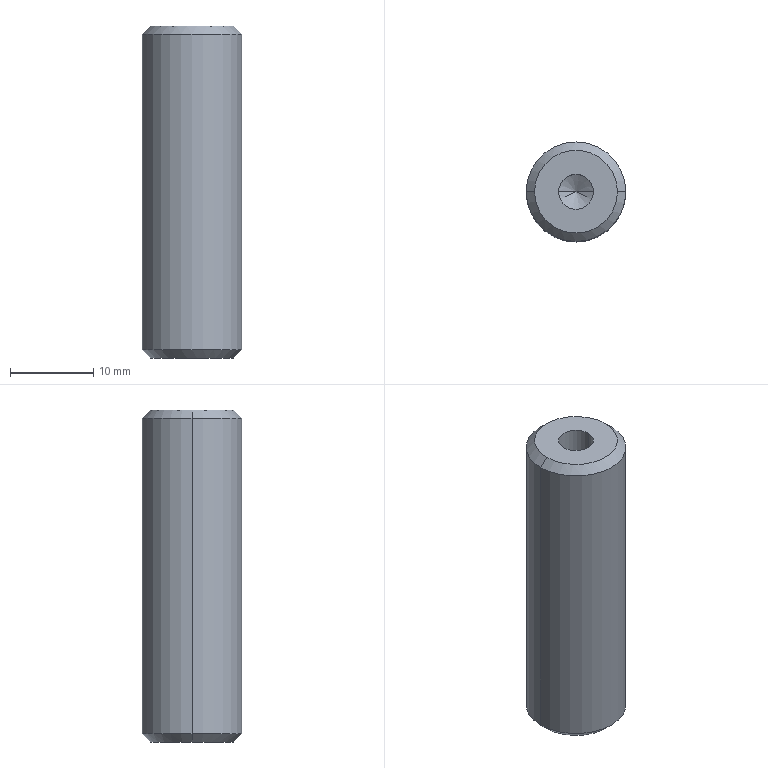Part | STEP file | PSFGT12-40-M5 | 1 solid | 12 faces | box 12 x 12 x 40 mm | volume 4311 mm3 | cone 6 | cylinder 4 | plane 2 | commonest cylinder face diameters 4.2 x2 12 x2
STEP:
#1=CARTESIAN_POINT('',(0.,0.,0.));
#2=DIRECTION('',(0.,0.,1.));
#3=DIRECTION('',(1.,0.,0.));
#4=AXIS2_PLACEMENT_3D('',#1,#2,#3);
#5=CARTESIAN_POINT('',(2.1,0.,27.6));
#6=VERTEX_POINT('',#5);
#7=CARTESIAN_POINT('',(2.1,0.,40.));
#8=VERTEX_POINT('',#7);
#9=CARTESIAN_POINT('',(2.1,0.,40.));
#10=DIRECTION('',(0.,0.,1.));
#11=VECTOR('',#10,1.);
#12=LINE('',#9,#11);
#13=CARTESIAN_POINT('',(0.,0.,40.));
#14=DIRECTION('',(0.,0.,1.));
#15=DIRECTION('',(1.,0.,0.));
#16=AXIS2_PLACEMENT_3D('',#13,#14,#15);
#17=CYLINDRICAL_SURFACE('',#16,2.1);
#18=CARTESIAN_POINT('',(6.283,0.));
#19=DIRECTION('',(0.,1.));
#20=VECTOR('',#19,1.);
#21=LINE('',#18,#20);
#22=(GEOMETRIC_REPRESENTATION_CONTEXT(2)PARAMETRIC_REPRESENTATION_CONTEXT()REPRESENTATION_CONTEXT('',''));
#23=DEFINITIONAL_REPRESENTATION('',(#21),#22);
#24=PCURVE('',#17,#23);
#25=CARTESIAN_POINT('',(0.,0.,40.));
#26=DIRECTION('',(0.,0.,1.));
#27=DIRECTION('',(1.,0.,0.));
#28=AXIS2_PLACEMENT_3D('',#25,#26,#27);
#29=CYLINDRICAL_SURFACE('',#28,2.1);
#30=CARTESIAN_POINT('',(0.,0.));
#31=DIRECTION('',(0.,1.));
#32=VECTOR('',#31,1.);
#33=LINE('',#30,#32);
#34=(GEOMETRIC_REPRESENTATION_CONTEXT(2)PARAMETRIC_REPRESENTATION_CONTEXT()REPRESENTATION_CONTEXT('',''));
#35=DEFINITIONAL_REPRESENTATION('',(#33),#34);
#36=PCURVE('',#29,#35);
#37=SURFACE_CURVE('',#12,(#24,#36),.PCURVE_S1.);
#38=EDGE_CURVE('',#6,#8,#37,.T.);
#39=ORIENTED_EDGE('',*,*,#38,.T.);
#40=CARTESIAN_POINT('',(-2.1,0.,40.));
#41=VERTEX_POINT('',#40);
#42=CARTESIAN_POINT('',(0.,0.,40.));
#43=DIRECTION('',(0.,0.,1.));
#44=DIRECTION('',(1.,0.,0.));
#45=AXIS2_PLACEMENT_3D('',#42,#43,#44);
#46=CIRCLE('',#45,2.1);
#47=CARTESIAN_POINT('',(0.,0.));
#48=DIRECTION('',(1.,0.));
#49=VECTOR('',#48,1.);
#50=LINE('',#47,#49);
#51=(GEOMETRIC_REPRESENTATION_CONTEXT(2)PARAMETRIC_REPRESENTATION_CONTEXT()REPRESENTATION_CONTEXT('',''));
#52=DEFINITIONAL_REPRESENTATION('',(#50),#51);
#53=PCURVE('',#17,#52);
#54=CARTESIAN_POINT('',(0.,0.,40.));
#55=DIRECTION('',(0.,0.,1.));
#56=DIRECTION('',(1.,0.,0.));
#57=AXIS2_PLACEMENT_3D('',#54,#55,#56);
#58=PLANE('',#57);
#59=CARTESIAN_POINT('',(0.,0.));
#60=DIRECTION('',(1.,0.));
#61=AXIS2_PLACEMENT_2D('',#59,#60);
#62=CIRCLE('',#61,2.1);
#63=(GEOMETRIC_REPRESENTATION_CONTEXT(2)PARAMETRIC_REPRESENTATION_CONTEXT()REPRESENTATION_CONTEXT('',''));
#64=DEFINITIONAL_REPRESENTATION('',(#62),#63);
#65=PCURVE('',#58,#64);
#66=SURFACE_CURVE('',#46,(#53,#65),.PCURVE_S1.);
#67=EDGE_CURVE('',#41,#8,#66,.T.);
#68=ORIENTED_EDGE('',*,*,#67,.F.);
#69=CARTESIAN_POINT('',(-2.1,0.,27.6));
#70=VERTEX_POINT('',#69);
#71=CARTESIAN_POINT('',(-2.1,0.,40.));
#72=DIRECTION('',(0.,0.,1.));
#73=VECTOR('',#72,1.);
#74=LINE('',#71,#73);
#75=CARTESIAN_POINT('',(3.142,0.));
#76=DIRECTION('',(0.,1.));
#77=VECTOR('',#76,1.);
#78=LINE('',#75,#77);
#79=(GEOMETRIC_REPRESENTATION_CONTEXT(2)PARAMETRIC_REPRESENTATION_CONTEXT()REPRESENTATION_CONTEXT('',''));
#80=DEFINITIONAL_REPRESENTATION('',(#78),#79);
#81=PCURVE('',#17,#80);
#82=CARTESIAN_POINT('',(3.142,0.));
#83=DIRECTION('',(0.,1.));
#84=VECTOR('',#83,1.);
#85=LINE('',#82,#84);
#86=(GEOMETRIC_REPRESENTATION_CONTEXT(2)PARAMETRIC_REPRESENTATION_CONTEXT()REPRESENTATION_CONTEXT('',''));
#87=DEFINITIONAL_REPRESENTATION('',(#85),#86);
#88=PCURVE('',#29,#87);
#89=SURFACE_CURVE('',#74,(#81,#88),.PCURVE_S1.);
#90=EDGE_CURVE('',#70,#41,#89,.T.);
#91=ORIENTED_EDGE('',*,*,#90,.F.);
#92=CARTESIAN_POINT('',(0.,0.,27.6));
#93=DIRECTION('',(0.,0.,1.));
#94=DIRECTION('',(1.,0.,0.));
#95=AXIS2_PLACEMENT_3D('',#92,#93,#94);
#96=CIRCLE('',#95,2.1);
#97=CARTESIAN_POINT('',(0.,-12.4));
#98=DIRECTION('',(1.,0.));
#99=VECTOR('',#98,1.);
#100=LINE('',#97,#99);
#101=(GEOMETRIC_REPRESENTATION_CONTEXT(2)PARAMETRIC_REPRESENTATION_CONTEXT()REPRESENTATION_CONTEXT('',''));
#102=DEFINITIONAL_REPRESENTATION('',(#100),#101);
#103=PCURVE('',#17,#102);
#104=CARTESIAN_POINT('',(0.,0.,27.6));
#105=DIRECTION('',(0.,0.,1.));
#106=DIRECTION('',(1.,0.,0.));
#107=AXIS2_PLACEMENT_3D('',#104,#105,#106);
#108=CONICAL_SURFACE('',#107,2.1,1.03);
#109=CARTESIAN_POINT('',(0.,0.));
#110=DIRECTION('',(1.,0.));
#111=VECTOR('',#110,1.);
#112=LINE('',#109,#111);
#113=(GEOMETRIC_REPRESENTATION_CONTEXT(2)PARAMETRIC_REPRESENTATION_CONTEXT()REPRESENTATION_CONTEXT('',''));
#114=DEFINITIONAL_REPRESENTATION('',(#112),#113);
#115=PCURVE('',#108,#114);
#116=SURFACE_CURVE('',#96,(#103,#115),.PCURVE_S1.);
#117=EDGE_CURVE('',#70,#6,#116,.T.);
#118=ORIENTED_EDGE('',*,*,#117,.T.);
#119=EDGE_LOOP('',(#39,#68,#91,#118));
#120=FACE_BOUND('',#119,.F.);
#121=ADVANCED_FACE('',(#120),#17,.F.);
#122=ORIENTED_EDGE('',*,*,#117,.F.);
#123=CARTESIAN_POINT('',(0.,0.,26.338));
#124=VERTEX_POINT('',#123);
#125=CARTESIAN_POINT('',(-2.1,0.,27.6));
#126=DIRECTION('',(-0.8572,0.,0.515));
#127=VECTOR('',#126,1.);
#128=LINE('',#125,#127);
#129=CARTESIAN_POINT('',(3.142,0.));
#130=DIRECTION('',(0.,1.));
#131=VECTOR('',#130,1.);
#132=LINE('',#129,#131);
#133=(GEOMETRIC_REPRESENTATION_CONTEXT(2)PARAMETRIC_REPRESENTATION_CONTEXT()REPRESENTATION_CONTEXT('',''));
#134=DEFINITIONAL_REPRESENTATION('',(#132),#133);
#135=PCURVE('',#108,#134);
#136=CARTESIAN_POINT('',(0.,0.,27.6));
#137=DIRECTION('',(0.,0.,1.));
#138=DIRECTION('',(1.,0.,0.));
#139=AXIS2_PLACEMENT_3D('',#136,#137,#138);
#140=CONICAL_SURFACE('',#139,2.1,1.03);
#141=CARTESIAN_POINT('',(3.142,0.));
#142=DIRECTION('',(0.,1.));
#143=VECTOR('',#142,1.);
#144=LINE('',#141,#143);
#145=(GEOMETRIC_REPRESENTATION_CONTEXT(2)PARAMETRIC_REPRESENTATION_CONTEXT()REPRESENTATION_CONTEXT('',''));
#146=DEFINITIONAL_REPRESENTATION('',(#144),#145);
#147=PCURVE('',#140,#146);
#148=SURFACE_CURVE('',#128,(#135,#147),.PCURVE_S1.);
#149=EDGE_CURVE('',#124,#70,#148,.T.);
#150=ORIENTED_EDGE('',*,*,#149,.F.);
#151=CARTESIAN_POINT('',(2.1,0.,27.6));
#152=DIRECTION('',(0.8572,0.,0.515));
#153=VECTOR('',#152,1.);
#154=LINE('',#151,#153);
#155=CARTESIAN_POINT('',(6.283,-1.262));
#156=CARTESIAN_POINT('',(6.283,-1.243));
#157=CARTESIAN_POINT('',(6.283,-1.204));
#158=CARTESIAN_POINT('',(6.283,-1.147));
#159=CARTESIAN_POINT('',(6.283,-1.09));
#160=CARTESIAN_POINT('',(6.283,-1.032));
#161=CARTESIAN_POINT('',(6.283,-0.975));
#162=CARTESIAN_POINT('',(6.283,-0.9177));
#163=CARTESIAN_POINT('',(6.283,-0.8603));
#164=CARTESIAN_POINT('',(6.283,-0.803));
#165=CARTESIAN_POINT('',(6.283,-0.7456));
#166=CARTESIAN_POINT('',(6.283,-0.6883));
#167=CARTESIAN_POINT('',(6.283,-0.6309));
#168=CARTESIAN_POINT('',(6.283,-0.5735));
#169=CARTESIAN_POINT('',(6.283,-0.5162));
#170=CARTESIAN_POINT('',(6.283,-0.4588));
#171=CARTESIAN_POINT('',(6.283,-0.4015));
#172=CARTESIAN_POINT('',(6.283,-0.3441));
#173=CARTESIAN_POINT('',(6.283,-0.2868));
#174=CARTESIAN_POINT('',(6.283,-0.2294));
#175=CARTESIAN_POINT('',(6.283,-0.1721));
#176=CARTESIAN_POINT('',(6.283,-0.1147));
#177=CARTESIAN_POINT('',(6.283,-0.05735));
#178=CARTESIAN_POINT('',(6.283,-0.01912));
#179=CARTESIAN_POINT('',(6.283,0.));
#180=B_SPLINE_CURVE_WITH_KNOTS('',3,(#155,#156,#157,#158,#159,#160,#161,#162,#163,#164,#165,#166,#167,#168,#169,#170,#171,#172,#173,#174,#175,#176,#177,#178,#179),.UNSPECIFIED.,.F.,.F.,(4,1,1,1,1,1,1,1,1,1,1,1,1,1,1,1,1,1,1,1,1,1,4),(-2.45,-2.339,-2.227,-2.116,-2.004,-1.893,-1.782,-1.67,-1.559,-1.448,-1.336,-1.225,-1.114,-1.002,-0.8909,-0.7795,-0.6682,-0.5568,-0.4454,-0.3341,-0.2227,-0.1114,0.),.UNSPECIFIED.);
#181=(GEOMETRIC_REPRESENTATION_CONTEXT(2)PARAMETRIC_REPRESENTATION_CONTEXT()REPRESENTATION_CONTEXT('',''));
#182=DEFINITIONAL_REPRESENTATION('',(#180),#181);
#183=PCURVE('',#108,#182);
#184=CARTESIAN_POINT('',(0.,-1.262));
#185=CARTESIAN_POINT('',(0.,-1.243));
#186=CARTESIAN_POINT('',(0.,-1.204));
#187=CARTESIAN_POINT('',(0.,-1.147));
#188=CARTESIAN_POINT('',(0.,-1.09));
#189=CARTESIAN_POINT('',(0.,-1.032));
#190=CARTESIAN_POINT('',(0.,-0.975));
#191=CARTESIAN_POINT('',(0.,-0.9177));
#192=CARTESIAN_POINT('',(0.,-0.8603));
#193=CARTESIAN_POINT('',(0.,-0.803));
#194=CARTESIAN_POINT('',(0.,-0.7456));
#195=CARTESIAN_POINT('',(0.,-0.6883));
#196=CARTESIAN_POINT('',(0.,-0.6309));
#197=CARTESIAN_POINT('',(0.,-0.5735));
#198=CARTESIAN_POINT('',(0.,-0.5162));
#199=CARTESIAN_POINT('',(0.,-0.4588));
#200=CARTESIAN_POINT('',(0.,-0.4015));
#201=CARTESIAN_POINT('',(0.,-0.3441));
#202=CARTESIAN_POINT('',(0.,-0.2868));
#203=CARTESIAN_POINT('',(0.,-0.2294));
#204=CARTESIAN_POINT('',(0.,-0.1721));
#205=CARTESIAN_POINT('',(0.,-0.1147));
#206=CARTESIAN_POINT('',(0.,-0.05735));
#207=CARTESIAN_POINT('',(0.,-0.01912));
#208=CARTESIAN_POINT('',(0.,0.));
#209=B_SPLINE_CURVE_WITH_KNOTS('',3,(#184,#185,#186,#187,#188,#189,#190,#191,#192,#193,#194,#195,#196,#197,#198,#199,#200,#201,#202,#203,#204,#205,#206,#207,#208),.UNSPECIFIED.,.F.,.F.,(4,1,1,1,1,1,1,1,1,1,1,1,1,1,1,1,1,1,1,1,1,1,4),(-2.45,-2.339,-2.227,-2.116,-2.004,-1.893,-1.782,-1.67,-1.559,-1.448,-1.336,-1.225,-1.114,-1.002,-0.8909,-0.7795,-0.6682,-0.5568,-0.4454,-0.3341,-0.2227,-0.1114,0.),.UNSPECIFIED.);
#210=(GEOMETRIC_REPRESENTATION_CONTEXT(2)PARAMETRIC_REPRESENTATION_CONTEXT()REPRESENTATION_CONTEXT('',''));
#211=DEFINITIONAL_REPRESENTATION('',(#209),#210);
#212=PCURVE('',#140,#211);
#213=SURFACE_CURVE('',#154,(#183,#212),.PCURVE_S1.);
#214=EDGE_CURVE('',#124,#6,#213,.T.);
#215=ORIENTED_EDGE('',*,*,#214,.T.);
#216=EDGE_LOOP('',(#122,#150,#215));
#217=FACE_BOUND('',#216,.F.);
#218=ADVANCED_FACE('',(#217),#108,.F.);
#219=CARTESIAN_POINT('',(5.,0.,40.));
#220=VERTEX_POINT('',#219);
#221=CARTESIAN_POINT('',(-5.,0.,40.));
#222=VERTEX_POINT('',#221);
#223=CARTESIAN_POINT('',(0.,0.,40.));
#224=DIRECTION('',(0.,0.,1.));
#225=DIRECTION('',(1.,0.,0.));
#226=AXIS2_PLACEMENT_3D('',#223,#224,#225);
#227=CIRCLE('',#226,5.);
#228=CARTESIAN_POINT('',(0.,0.,40.));
#229=DIRECTION('',(0.,0.,-1.));
#230=DIRECTION('',(-1.,0.,0.));
#231=AXIS2_PLACEMENT_3D('',#228,#229,#230);
#232=CONICAL_SURFACE('',#231,5.,0.7854);
#233=CARTESIAN_POINT('',(3.142,0.));
#234=DIRECTION('',(-1.,0.));
#235=VECTOR('',#234,1.);
#236=LINE('',#233,#235);
#237=(GEOMETRIC_REPRESENTATION_CONTEXT(2)PARAMETRIC_REPRESENTATION_CONTEXT()REPRESENTATION_CONTEXT('',''));
#238=DEFINITIONAL_REPRESENTATION('',(#236),#237);
#239=PCURVE('',#232,#238);
#240=CARTESIAN_POINT('',(0.,0.));
#241=DIRECTION('',(1.,0.));
#242=AXIS2_PLACEMENT_2D('',#240,#241);
#243=CIRCLE('',#242,5.);
#244=(GEOMETRIC_REPRESENTATION_CONTEXT(2)PARAMETRIC_REPRESENTATION_CONTEXT()REPRESENTATION_CONTEXT('',''));
#245=DEFINITIONAL_REPRESENTATION('',(#243),#244);
#246=PCURVE('',#58,#245);
#247=SURFACE_CURVE('',#227,(#239,#246),.PCURVE_S1.);
#248=EDGE_CURVE('',#220,#222,#247,.T.);
#249=ORIENTED_EDGE('',*,*,#248,.F.);
#250=CARTESIAN_POINT('',(6.,0.,39.));
#251=VERTEX_POINT('',#250);
#252=CARTESIAN_POINT('',(5.,0.,40.));
#253=DIRECTION('',(0.7071,0.,-0.7071));
#254=VECTOR('',#253,1.);
#255=LINE('',#252,#254);
#256=CARTESIAN_POINT('',(3.142,0.));
#257=DIRECTION('',(0.,1.));
#258=VECTOR('',#257,1.);
#259=LINE('',#256,#258);
#260=(GEOMETRIC_REPRESENTATION_CONTEXT(2)PARAMETRIC_REPRESENTATION_CONTEXT()REPRESENTATION_CONTEXT('',''));
#261=DEFINITIONAL_REPRESENTATION('',(#259),#260);
#262=PCURVE('',#232,#261);
#263=CARTESIAN_POINT('',(0.,0.,40.));
#264=DIRECTION('',(0.,0.,-1.));
#265=DIRECTION('',(-1.,0.,0.));
#266=AXIS2_PLACEMENT_3D('',#263,#264,#265);
#267=CONICAL_SURFACE('',#266,5.,0.7854);
#268=CARTESIAN_POINT('',(3.142,0.));
#269=DIRECTION('',(0.,1.));
#270=VECTOR('',#269,1.);
#271=LINE('',#268,#270);
#272=(GEOMETRIC_REPRESENTATION_CONTEXT(2)PARAMETRIC_REPRESENTATION_CONTEXT()REPRESENTATION_CONTEXT('',''));
#273=DEFINITIONAL_REPRESENTATION('',(#271),#272);
#274=PCURVE('',#267,#273);
#275=SURFACE_CURVE('',#255,(#262,#274),.PCURVE_S1.);
#276=EDGE_CURVE('',#220,#251,#275,.T.);
#277=ORIENTED_EDGE('',*,*,#276,.T.);
#278=CARTESIAN_POINT('',(-6.,0.,39.));
#279=VERTEX_POINT('',#278);
#280=CARTESIAN_POINT('',(0.,0.,39.));
#281=DIRECTION('',(0.,0.,-1.));
#282=DIRECTION('',(1.,0.,0.));
#283=AXIS2_PLACEMENT_3D('',#280,#281,#282);
#284=CIRCLE('',#283,6.);
#285=CARTESIAN_POINT('',(-3.142,1.));
#286=DIRECTION('',(1.,0.));
#287=VECTOR('',#286,1.);
#288=LINE('',#285,#287);
#289=(GEOMETRIC_REPRESENTATION_CONTEXT(2)PARAMETRIC_REPRESENTATION_CONTEXT()REPRESENTATION_CONTEXT('',''));
#290=DEFINITIONAL_REPRESENTATION('',(#288),#289);
#291=PCURVE('',#232,#290);
#292=CARTESIAN_POINT('',(0.,0.,40.));
#293=DIRECTION('',(0.,0.,-1.));
#294=DIRECTION('',(-1.,0.,0.));
#295=AXIS2_PLACEMENT_3D('',#292,#293,#294);
#296=CYLINDRICAL_SURFACE('',#295,6.);
#297=CARTESIAN_POINT('',(-3.142,1.));
#298=DIRECTION('',(1.,0.));
#299=VECTOR('',#298,1.);
#300=LINE('',#297,#299);
#301=(GEOMETRIC_REPRESENTATION_CONTEXT(2)PARAMETRIC_REPRESENTATION_CONTEXT()REPRESENTATION_CONTEXT('',''));
#302=DEFINITIONAL_REPRESENTATION('',(#300),#301);
#303=PCURVE('',#296,#302);
#304=SURFACE_CURVE('',#284,(#291,#303),.PCURVE_S1.);
#305=EDGE_CURVE('',#279,#251,#304,.T.);
#306=ORIENTED_EDGE('',*,*,#305,.F.);
#307=CARTESIAN_POINT('',(-5.,0.,40.));
#308=DIRECTION('',(-0.7071,0.,-0.7071));
#309=VECTOR('',#308,1.);
#310=LINE('',#307,#309);
#311=CARTESIAN_POINT('',(0.,0.));
#312=DIRECTION('',(0.,1.));
#313=VECTOR('',#312,1.);
#314=LINE('',#311,#313);
#315=(GEOMETRIC_REPRESENTATION_CONTEXT(2)PARAMETRIC_REPRESENTATION_CONTEXT()REPRESENTATION_CONTEXT('',''));
#316=DEFINITIONAL_REPRESENTATION('',(#314),#315);
#317=PCURVE('',#232,#316);
#318=CARTESIAN_POINT('',(6.283,0.));
#319=DIRECTION('',(0.,1.));
#320=VECTOR('',#319,1.);
#321=LINE('',#318,#320);
#322=(GEOMETRIC_REPRESENTATION_CONTEXT(2)PARAMETRIC_REPRESENTATION_CONTEXT()REPRESENTATION_CONTEXT('',''));
#323=DEFINITIONAL_REPRESENTATION('',(#321),#322);
#324=PCURVE('',#267,#323);
#325=SURFACE_CURVE('',#310,(#317,#324),.PCURVE_S1.);
#326=EDGE_CURVE('',#222,#279,#325,.T.);
#327=ORIENTED_EDGE('',*,*,#326,.F.);
#328=EDGE_LOOP('',(#249,#277,#306,#327));
#329=FACE_BOUND('',#328,.T.);
#330=ADVANCED_FACE('',(#329),#232,.T.);
#331=CARTESIAN_POINT('',(-5.,0.,0.));
#332=VERTEX_POINT('',#331);
#333=CARTESIAN_POINT('',(5.,0.,0.));
#334=VERTEX_POINT('',#333);
#335=CARTESIAN_POINT('',(0.,0.,0.));
#336=DIRECTION('',(0.,0.,-1.));
#337=DIRECTION('',(1.,0.,0.));
#338=AXIS2_PLACEMENT_3D('',#335,#336,#337);
#339=CIRCLE('',#338,5.);
#340=CARTESIAN_POINT('',(0.,0.,1.));
#341=DIRECTION('',(0.,0.,1.));
#342=DIRECTION('',(1.,0.,0.));
#343=AXIS2_PLACEMENT_3D('',#340,#341,#342);
#344=CONICAL_SURFACE('',#343,6.,0.7854);
#345=CARTESIAN_POINT('',(6.283,-1.));
#346=DIRECTION('',(-1.,0.));
#347=VECTOR('',#346,1.);
#348=LINE('',#345,#347);
#349=(GEOMETRIC_REPRESENTATION_CONTEXT(2)PARAMETRIC_REPRESENTATION_CONTEXT()REPRESENTATION_CONTEXT('',''));
#350=DEFINITIONAL_REPRESENTATION('',(#348),#349);
#351=PCURVE('',#344,#350);
#352=CARTESIAN_POINT('',(0.,0.,0.));
#353=DIRECTION('',(0.,0.,1.));
#354=DIRECTION('',(1.,0.,0.));
#355=AXIS2_PLACEMENT_3D('',#352,#353,#354);
#356=PLANE('',#355);
#357=CARTESIAN_POINT('',(5.,0.));
#358=CARTESIAN_POINT('',(5.,-8.66));
#359=CARTESIAN_POINT('',(-2.5,-4.33));
#360=CARTESIAN_POINT('',(-10.,0.));
#361=CARTESIAN_POINT('',(-2.5,4.33));
#362=CARTESIAN_POINT('',(5.,8.66));
#363=CARTESIAN_POINT('',(5.,0.));
#364=(BOUNDED_CURVE()B_SPLINE_CURVE(2,(#357,#358,#359,#360,#361,#362,#363),.UNSPECIFIED.,.T.,.F.)B_SPLINE_CURVE_WITH_KNOTS((1,2,2,2,2,1),(-2.094,0.,2.094,4.189,6.283,8.378),.UNSPECIFIED.)CURVE()GEOMETRIC_REPRESENTATION_ITEM()RATIONAL_B_SPLINE_CURVE((1.,0.5,1.,0.5,1.,0.5,1.))REPRESENTATION_ITEM(''));
#365=(GEOMETRIC_REPRESENTATION_CONTEXT(2)PARAMETRIC_REPRESENTATION_CONTEXT()REPRESENTATION_CONTEXT('',''));
#366=DEFINITIONAL_REPRESENTATION('',(#364),#365);
#367=PCURVE('',#356,#366);
#368=SURFACE_CURVE('',#339,(#351,#367),.PCURVE_S1.);
#369=EDGE_CURVE('',#332,#334,#368,.T.);
#370=ORIENTED_EDGE('',*,*,#369,.F.);
#371=CARTESIAN_POINT('',(-6.,0.,1.));
#372=VERTEX_POINT('',#371);
#373=CARTESIAN_POINT('',(-6.,0.,1.));
#374=DIRECTION('',(-0.7071,0.,0.7071));
#375=VECTOR('',#374,1.);
#376=LINE('',#373,#375);
#377=CARTESIAN_POINT('',(3.142,0.));
#378=DIRECTION('',(0.,1.));
#379=VECTOR('',#378,1.);
#380=LINE('',#377,#379);
#381=(GEOMETRIC_REPRESENTATION_CONTEXT(2)PARAMETRIC_REPRESENTATION_CONTEXT()REPRESENTATION_CONTEXT('',''));
#382=DEFINITIONAL_REPRESENTATION('',(#380),#381);
#383=PCURVE('',#344,#382);
#384=CARTESIAN_POINT('',(0.,0.,1.));
#385=DIRECTION('',(0.,0.,1.));
#386=DIRECTION('',(1.,0.,0.));
#387=AXIS2_PLACEMENT_3D('',#384,#385,#386);
#388=CONICAL_SURFACE('',#387,6.,0.7854);
#389=CARTESIAN_POINT('',(3.142,0.));
#390=DIRECTION('',(0.,1.));
#391=VECTOR('',#390,1.);
#392=LINE('',#389,#391);
#393=(GEOMETRIC_REPRESENTATION_CONTEXT(2)PARAMETRIC_REPRESENTATION_CONTEXT()REPRESENTATION_CONTEXT('',''));
#394=DEFINITIONAL_REPRESENTATION('',(#392),#393);
#395=PCURVE('',#388,#394);
#396=SURFACE_CURVE('',#376,(#383,#395),.PCURVE_S1.);
#397=EDGE_CURVE('',#332,#372,#396,.T.);
#398=ORIENTED_EDGE('',*,*,#397,.T.);
#399=CARTESIAN_POINT('',(6.,0.,1.));
#400=VERTEX_POINT('',#399);
#401=CARTESIAN_POINT('',(0.,0.,1.));
#402=DIRECTION('',(0.,0.,1.));
#403=DIRECTION('',(1.,0.,0.));
#404=AXIS2_PLACEMENT_3D('',#401,#402,#403);
#405=CIRCLE('',#404,6.);
#406=CARTESIAN_POINT('',(0.,0.));
#407=DIRECTION('',(1.,0.));
#408=VECTOR('',#407,1.);
#409=LINE('',#406,#408);
#410=(GEOMETRIC_REPRESENTATION_CONTEXT(2)PARAMETRIC_REPRESENTATION_CONTEXT()REPRESENTATION_CONTEXT('',''));
#411=DEFINITIONAL_REPRESENTATION('',(#409),#410);
#412=PCURVE('',#344,#411);
#413=CARTESIAN_POINT('',(3.142,39.));
#414=DIRECTION('',(-1.,0.));
#415=VECTOR('',#414,1.);
#416=LINE('',#413,#415);
#417=(GEOMETRIC_REPRESENTATION_CONTEXT(2)PARAMETRIC_REPRESENTATION_CONTEXT()REPRESENTATION_CONTEXT('',''));
#418=DEFINITIONAL_REPRESENTATION('',(#416),#417);
#419=PCURVE('',#296,#418);
#420=SURFACE_CURVE('',#405,(#412,#419),.PCURVE_S1.);
#421=EDGE_CURVE('',#400,#372,#420,.T.);
#422=ORIENTED_EDGE('',*,*,#421,.F.);
#423=CARTESIAN_POINT('',(6.,0.,1.));
#424=DIRECTION('',(0.7071,0.,0.7071));
#425=VECTOR('',#424,1.);
#426=LINE('',#423,#425);
#427=CARTESIAN_POINT('',(0.,0.));
#428=DIRECTION('',(0.,1.));
#429=VECTOR('',#428,1.);
#430=LINE('',#427,#429);
#431=(GEOMETRIC_REPRESENTATION_CONTEXT(2)PARAMETRIC_REPRESENTATION_CONTEXT()REPRESENTATION_CONTEXT('',''));
#432=DEFINITIONAL_REPRESENTATION('',(#430),#431);
#433=PCURVE('',#344,#432);
#434=CARTESIAN_POINT('',(6.283,0.));
#435=DIRECTION('',(0.,1.));
#436=VECTOR('',#435,1.);
#437=LINE('',#434,#436);
#438=(GEOMETRIC_REPRESENTATION_CONTEXT(2)PARAMETRIC_REPRESENTATION_CONTEXT()REPRESENTATION_CONTEXT('',''));
#439=DEFINITIONAL_REPRESENTATION('',(#437),#438);
#440=PCURVE('',#388,#439);
#441=SURFACE_CURVE('',#426,(#433,#440),.PCURVE_S1.);
#442=EDGE_CURVE('',#334,#400,#441,.T.);
#443=ORIENTED_EDGE('',*,*,#442,.F.);
#444=EDGE_LOOP('',(#370,#398,#422,#443));
#445=FACE_BOUND('',#444,.T.);
#446=ADVANCED_FACE('',(#445),#344,.T.);
#447=ORIENTED_EDGE('',*,*,#305,.T.);
#448=CARTESIAN_POINT('',(6.,0.,40.));
#449=DIRECTION('',(0.,0.,-1.));
#450=VECTOR('',#449,1.);
#451=LINE('',#448,#450);
#452=CARTESIAN_POINT('',(3.142,0.));
#453=DIRECTION('',(0.,1.));
#454=VECTOR('',#453,1.);
#455=LINE('',#452,#454);
#456=(GEOMETRIC_REPRESENTATION_CONTEXT(2)PARAMETRIC_REPRESENTATION_CONTEXT()REPRESENTATION_CONTEXT('',''));
#457=DEFINITIONAL_REPRESENTATION('',(#455),#456);
#458=PCURVE('',#296,#457);
#459=CARTESIAN_POINT('',(0.,0.,40.));
#460=DIRECTION('',(0.,0.,-1.));
#461=DIRECTION('',(-1.,0.,0.));
#462=AXIS2_PLACEMENT_3D('',#459,#460,#461);
#463=CYLINDRICAL_SURFACE('',#462,6.);
#464=CARTESIAN_POINT('',(3.142,0.));
#465=DIRECTION('',(0.,1.));
#466=VECTOR('',#465,1.);
#467=LINE('',#464,#466);
#468=(GEOMETRIC_REPRESENTATION_CONTEXT(2)PARAMETRIC_REPRESENTATION_CONTEXT()REPRESENTATION_CONTEXT('',''));
#469=DEFINITIONAL_REPRESENTATION('',(#467),#468);
#470=PCURVE('',#463,#469);
#471=SURFACE_CURVE('',#451,(#458,#470),.PCURVE_S1.);
#472=EDGE_CURVE('',#251,#400,#471,.T.);
#473=ORIENTED_EDGE('',*,*,#472,.T.);
#474=ORIENTED_EDGE('',*,*,#421,.T.);
#475=CARTESIAN_POINT('',(-6.,0.,40.));
#476=DIRECTION('',(0.,0.,-1.));
#477=VECTOR('',#476,1.);
#478=LINE('',#475,#477);
#479=CARTESIAN_POINT('',(0.,0.));
#480=DIRECTION('',(0.,1.));
#481=VECTOR('',#480,1.);
#482=LINE('',#479,#481);
#483=(GEOMETRIC_REPRESENTATION_CONTEXT(2)PARAMETRIC_REPRESENTATION_CONTEXT()REPRESENTATION_CONTEXT('',''));
#484=DEFINITIONAL_REPRESENTATION('',(#482),#483);
#485=PCURVE('',#296,#484);
#486=CARTESIAN_POINT('',(6.283,0.));
#487=DIRECTION('',(0.,1.));
#488=VECTOR('',#487,1.);
#489=LINE('',#486,#488);
#490=(GEOMETRIC_REPRESENTATION_CONTEXT(2)PARAMETRIC_REPRESENTATION_CONTEXT()REPRESENTATION_CONTEXT('',''));
#491=DEFINITIONAL_REPRESENTATION('',(#489),#490);
#492=PCURVE('',#463,#491);
#493=SURFACE_CURVE('',#478,(#485,#492),.PCURVE_S1.);
#494=EDGE_CURVE('',#279,#372,#493,.T.);
#495=ORIENTED_EDGE('',*,*,#494,.F.);
#496=EDGE_LOOP('',(#447,#473,#474,#495));
#497=FACE_BOUND('',#496,.T.);
#498=ADVANCED_FACE('',(#497),#296,.T.);
#499=ORIENTED_EDGE('',*,*,#472,.F.);
#500=CARTESIAN_POINT('',(0.,0.,39.));
#501=DIRECTION('',(0.,0.,-1.));
#502=DIRECTION('',(1.,0.,0.));
#503=AXIS2_PLACEMENT_3D('',#500,#501,#502);
#504=CIRCLE('',#503,6.);
#505=CARTESIAN_POINT('',(3.142,1.));
#506=DIRECTION('',(1.,0.));
#507=VECTOR('',#506,1.);
#508=LINE('',#505,#507);
#509=(GEOMETRIC_REPRESENTATION_CONTEXT(2)PARAMETRIC_REPRESENTATION_CONTEXT()REPRESENTATION_CONTEXT('',''));
#510=DEFINITIONAL_REPRESENTATION('',(#508),#509);
#511=PCURVE('',#463,#510);
#512=CARTESIAN_POINT('',(3.142,1.));
#513=DIRECTION('',(1.,0.));
#514=VECTOR('',#513,1.);
#515=LINE('',#512,#514);
#516=(GEOMETRIC_REPRESENTATION_CONTEXT(2)PARAMETRIC_REPRESENTATION_CONTEXT()REPRESENTATION_CONTEXT('',''));
#517=DEFINITIONAL_REPRESENTATION('',(#515),#516);
#518=PCURVE('',#267,#517);
#519=SURFACE_CURVE('',#504,(#511,#518),.PCURVE_S1.);
#520=EDGE_CURVE('',#251,#279,#519,.T.);
#521=ORIENTED_EDGE('',*,*,#520,.T.);
#522=ORIENTED_EDGE('',*,*,#494,.T.);
#523=CARTESIAN_POINT('',(0.,0.,1.));
#524=DIRECTION('',(0.,0.,1.));
#525=DIRECTION('',(1.,0.,0.));
#526=AXIS2_PLACEMENT_3D('',#523,#524,#525);
#527=CIRCLE('',#526,6.);
#528=CARTESIAN_POINT('',(9.425,39.));
#529=DIRECTION('',(-1.,0.));
#530=VECTOR('',#529,1.);
#531=LINE('',#528,#530);
#532=(GEOMETRIC_REPRESENTATION_CONTEXT(2)PARAMETRIC_REPRESENTATION_CONTEXT()REPRESENTATION_CONTEXT('',''));
#533=DEFINITIONAL_REPRESENTATION('',(#531),#532);
#534=PCURVE('',#463,#533);
#535=CARTESIAN_POINT('',(0.,0.));
#536=DIRECTION('',(1.,0.));
#537=VECTOR('',#536,1.);
#538=LINE('',#535,#537);
#539=(GEOMETRIC_REPRESENTATION_CONTEXT(2)PARAMETRIC_REPRESENTATION_CONTEXT()REPRESENTATION_CONTEXT('',''));
#540=DEFINITIONAL_REPRESENTATION('',(#538),#539);
#541=PCURVE('',#388,#540);
#542=SURFACE_CURVE('',#527,(#534,#541),.PCURVE_S1.);
#543=EDGE_CURVE('',#372,#400,#542,.T.);
#544=ORIENTED_EDGE('',*,*,#543,.T.);
#545=EDGE_LOOP('',(#499,#521,#522,#544));
#546=FACE_BOUND('',#545,.T.);
#547=ADVANCED_FACE('',(#546),#463,.T.);
#548=CARTESIAN_POINT('',(0.,0.,40.));
#549=DIRECTION('',(0.,0.,1.));
#550=DIRECTION('',(1.,0.,0.));
#551=AXIS2_PLACEMENT_3D('',#548,#549,#550);
#552=CIRCLE('',#551,2.1);
#553=CARTESIAN_POINT('',(0.,0.));
#554=DIRECTION('',(1.,0.));
#555=AXIS2_PLACEMENT_2D('',#553,#554);
#556=CIRCLE('',#555,2.1);
#557=(GEOMETRIC_REPRESENTATION_CONTEXT(2)PARAMETRIC_REPRESENTATION_CONTEXT()REPRESENTATION_CONTEXT('',''));
#558=DEFINITIONAL_REPRESENTATION('',(#556),#557);
#559=PCURVE('',#58,#558);
#560=CARTESIAN_POINT('',(0.,0.));
#561=DIRECTION('',(1.,0.));
#562=VECTOR('',#561,1.);
#563=LINE('',#560,#562);
#564=(GEOMETRIC_REPRESENTATION_CONTEXT(2)PARAMETRIC_REPRESENTATION_CONTEXT()REPRESENTATION_CONTEXT('',''));
#565=DEFINITIONAL_REPRESENTATION('',(#563),#564);
#566=PCURVE('',#29,#565);
#567=SURFACE_CURVE('',#552,(#559,#566),.PCURVE_S1.);
#568=EDGE_CURVE('',#8,#41,#567,.T.);
#569=ORIENTED_EDGE('',*,*,#568,.F.);
#570=ORIENTED_EDGE('',*,*,#67,.F.);
#571=EDGE_LOOP('',(#569,#570));
#572=FACE_BOUND('',#571,.T.);
#573=CARTESIAN_POINT('',(0.,0.,40.));
#574=DIRECTION('',(0.,0.,1.));
#575=DIRECTION('',(1.,0.,0.));
#576=AXIS2_PLACEMENT_3D('',#573,#574,#575);
#577=CIRCLE('',#576,5.);
#578=CARTESIAN_POINT('',(0.,0.));
#579=DIRECTION('',(1.,0.));
#580=AXIS2_PLACEMENT_2D('',#578,#579);
#581=CIRCLE('',#580,5.);
#582=(GEOMETRIC_REPRESENTATION_CONTEXT(2)PARAMETRIC_REPRESENTATION_CONTEXT()REPRESENTATION_CONTEXT('',''));
#583=DEFINITIONAL_REPRESENTATION('',(#581),#582);
#584=PCURVE('',#58,#583);
#585=CARTESIAN_POINT('',(9.425,0.));
#586=DIRECTION('',(-1.,0.));
#587=VECTOR('',#586,1.);
#588=LINE('',#585,#587);
#589=(GEOMETRIC_REPRESENTATION_CONTEXT(2)PARAMETRIC_REPRESENTATION_CONTEXT()REPRESENTATION_CONTEXT('',''));
#590=DEFINITIONAL_REPRESENTATION('',(#588),#589);
#591=PCURVE('',#267,#590);
#592=SURFACE_CURVE('',#577,(#584,#591),.PCURVE_S1.);
#593=EDGE_CURVE('',#222,#220,#592,.T.);
#594=ORIENTED_EDGE('',*,*,#593,.T.);
#595=ORIENTED_EDGE('',*,*,#248,.T.);
#596=EDGE_LOOP('',(#594,#595));
#597=FACE_BOUND('',#596,.T.);
#598=ADVANCED_FACE('',(#572,#597),#58,.T.);
#599=CARTESIAN_POINT('',(0.,0.,0.));
#600=DIRECTION('',(0.,0.,-1.));
#601=DIRECTION('',(1.,0.,0.));
#602=AXIS2_PLACEMENT_3D('',#599,#600,#601);
#603=CIRCLE('',#602,5.);
#604=CARTESIAN_POINT('',(5.,0.));
#605=CARTESIAN_POINT('',(5.,-8.66));
#606=CARTESIAN_POINT('',(-2.5,-4.33));
#607=CARTESIAN_POINT('',(-10.,0.));
#608=CARTESIAN_POINT('',(-2.5,4.33));
#609=CARTESIAN_POINT('',(5.,8.66));
#610=CARTESIAN_POINT('',(5.,0.));
#611=(BOUNDED_CURVE()B_SPLINE_CURVE(2,(#604,#605,#606,#607,#608,#609,#610),.UNSPECIFIED.,.T.,.F.)B_SPLINE_CURVE_WITH_KNOTS((1,2,2,2,2,1),(-2.094,0.,2.094,4.189,6.283,8.378),.UNSPECIFIED.)CURVE()GEOMETRIC_REPRESENTATION_ITEM()RATIONAL_B_SPLINE_CURVE((1.,0.5,1.,0.5,1.,0.5,1.))REPRESENTATION_ITEM(''));
#612=(GEOMETRIC_REPRESENTATION_CONTEXT(2)PARAMETRIC_REPRESENTATION_CONTEXT()REPRESENTATION_CONTEXT('',''));
#613=DEFINITIONAL_REPRESENTATION('',(#611),#612);
#614=PCURVE('',#356,#613);
#615=CARTESIAN_POINT('',(6.283,-1.));
#616=DIRECTION('',(-1.,0.));
#617=VECTOR('',#616,1.);
#618=LINE('',#615,#617);
#619=(GEOMETRIC_REPRESENTATION_CONTEXT(2)PARAMETRIC_REPRESENTATION_CONTEXT()REPRESENTATION_CONTEXT('',''));
#620=DEFINITIONAL_REPRESENTATION('',(#618),#619);
#621=PCURVE('',#388,#620);
#622=SURFACE_CURVE('',#603,(#614,#621),.PCURVE_S1.);
#623=EDGE_CURVE('',#334,#332,#622,.T.);
#624=ORIENTED_EDGE('',*,*,#623,.T.);
#625=ORIENTED_EDGE('',*,*,#369,.T.);
#626=EDGE_LOOP('',(#624,#625));
#627=FACE_BOUND('',#626,.T.);
#628=ADVANCED_FACE('',(#627),#356,.F.);
#629=ORIENTED_EDGE('',*,*,#397,.F.);
#630=ORIENTED_EDGE('',*,*,#623,.F.);
#631=ORIENTED_EDGE('',*,*,#442,.T.);
#632=ORIENTED_EDGE('',*,*,#543,.F.);
#633=EDGE_LOOP('',(#629,#630,#631,#632));
#634=FACE_BOUND('',#633,.T.);
#635=ADVANCED_FACE('',(#634),#388,.T.);
#636=ORIENTED_EDGE('',*,*,#276,.F.);
#637=ORIENTED_EDGE('',*,*,#593,.F.);
#638=ORIENTED_EDGE('',*,*,#326,.T.);
#639=ORIENTED_EDGE('',*,*,#520,.F.);
#640=EDGE_LOOP('',(#636,#637,#638,#639));
#641=FACE_BOUND('',#640,.T.);
#642=ADVANCED_FACE('',(#641),#267,.T.);
#643=CARTESIAN_POINT('',(0.,0.,27.6));
#644=DIRECTION('',(0.,0.,1.));
#645=DIRECTION('',(1.,0.,0.));
#646=AXIS2_PLACEMENT_3D('',#643,#644,#645);
#647=CIRCLE('',#646,2.1);
#648=CARTESIAN_POINT('',(0.,0.));
#649=DIRECTION('',(1.,0.));
#650=VECTOR('',#649,1.);
#651=LINE('',#648,#650);
#652=(GEOMETRIC_REPRESENTATION_CONTEXT(2)PARAMETRIC_REPRESENTATION_CONTEXT()REPRESENTATION_CONTEXT('',''));
#653=DEFINITIONAL_REPRESENTATION('',(#651),#652);
#654=PCURVE('',#140,#653);
#655=CARTESIAN_POINT('',(0.,-12.4));
#656=DIRECTION('',(1.,0.));
#657=VECTOR('',#656,1.);
#658=LINE('',#655,#657);
#659=(GEOMETRIC_REPRESENTATION_CONTEXT(2)PARAMETRIC_REPRESENTATION_CONTEXT()REPRESENTATION_CONTEXT('',''));
#660=DEFINITIONAL_REPRESENTATION('',(#658),#659);
#661=PCURVE('',#29,#660);
#662=SURFACE_CURVE('',#647,(#654,#661),.PCURVE_S1.);
#663=EDGE_CURVE('',#6,#70,#662,.T.);
#664=ORIENTED_EDGE('',*,*,#663,.F.);
#665=ORIENTED_EDGE('',*,*,#214,.F.);
#666=ORIENTED_EDGE('',*,*,#149,.T.);
#667=EDGE_LOOP('',(#664,#665,#666));
#668=FACE_BOUND('',#667,.F.);
#669=ADVANCED_FACE('',(#668),#140,.F.);
#670=ORIENTED_EDGE('',*,*,#568,.F.);
#671=ORIENTED_EDGE('',*,*,#38,.F.);
#672=ORIENTED_EDGE('',*,*,#663,.T.);
#673=ORIENTED_EDGE('',*,*,#90,.T.);
#674=EDGE_LOOP('',(#670,#671,#672,#673));
#675=FACE_BOUND('',#674,.F.);
#676=ADVANCED_FACE('',(#675),#29,.F.);
#677=CLOSED_SHELL('',(#121,#218,#330,#446,#498,#547,#598,#628,#635,#642,#669,#676));
#678=MANIFOLD_SOLID_BREP('',#677);
#679=(LENGTH_UNIT()NAMED_UNIT(*)SI_UNIT(.MILLI.,.METRE.));
#680=UNCERTAINTY_MEASURE_WITH_UNIT(LENGTH_MEASURE(0.0000001),#679,'','');
#681=(NAMED_UNIT(*)PLANE_ANGLE_UNIT()SI_UNIT($,.RADIAN.));
#682=(NAMED_UNIT(*)SI_UNIT($,.STERADIAN.)SOLID_ANGLE_UNIT());
#683=(GEOMETRIC_REPRESENTATION_CONTEXT(3)GLOBAL_UNCERTAINTY_ASSIGNED_CONTEXT((#680))GLOBAL_UNIT_ASSIGNED_CONTEXT((#679,#681,#682))REPRESENTATION_CONTEXT('',''));
#684=ADVANCED_BREP_SHAPE_REPRESENTATION('',(#4,#678),#683);